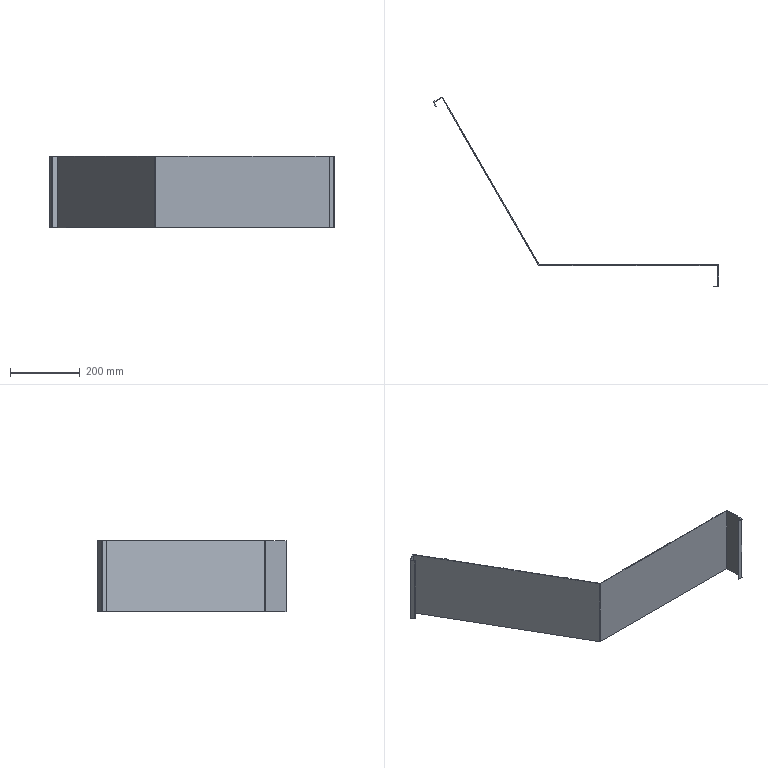Part | STEP file | zh003 | 1 solid | 56 faces | box 815.204 x 542.52 x 205 mm | volume 479740 mm3 | plane 44 | cylinder 12 | commonest cylinder face diameters 1 x6 5 x6